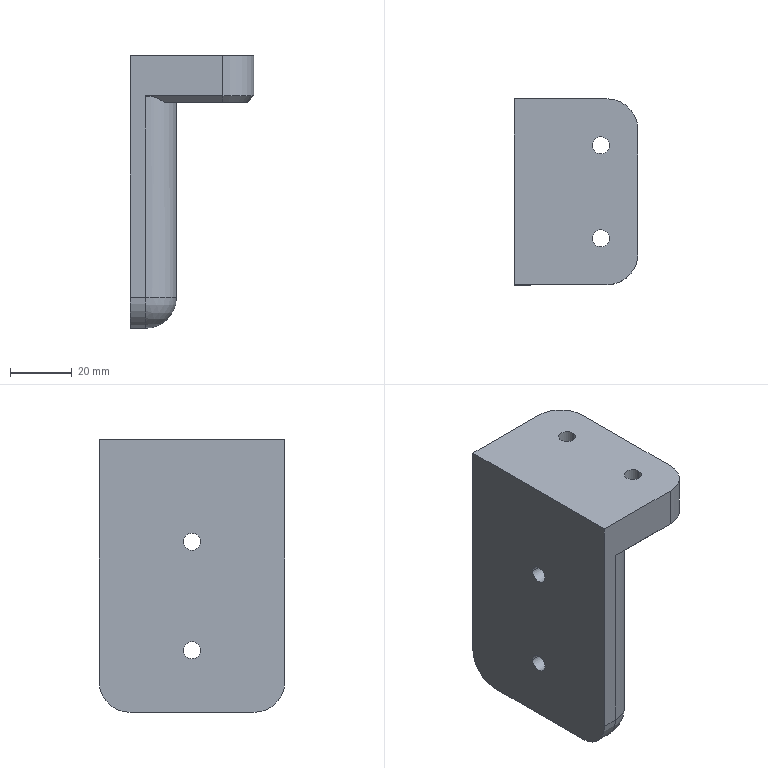Part | NX | features BREP 1 | 1 solid | 42 faces | box 40 x 60 x 88 mm | volume 93544 mm3 | cylinder 23 | plane 15 | cone 2 | sphere 2 | commonest cylinder face diameters 5.5 x8 9.5 x8 20 x7
STEP:
#1=CARTESIAN_POINT('',(30.,0.,-13.));
#2=VERTEX_POINT('',#1);
#3=CARTESIAN_POINT('',(30.,0.,0.));
#4=VERTEX_POINT('',#3);
#5=CARTESIAN_POINT('',(30.,0.,-13.));
#6=DIRECTION('',(0.000000001,0.,1.));
#7=VECTOR('',#6,1000.);
#8=LINE('',#5,#7);
#9=EDGE_CURVE('',#2,#4,#8,.T.);
#10=ORIENTED_EDGE('',*,*,#9,.T.);
#11=CARTESIAN_POINT('',(0.,0.,0.));
#12=VERTEX_POINT('',#11);
#13=CARTESIAN_POINT('',(0.,0.,0.));
#14=DIRECTION('',(1.,0.,0.));
#15=VECTOR('',#14,1000.);
#16=LINE('',#13,#15);
#17=EDGE_CURVE('',#12,#4,#16,.T.);
#18=ORIENTED_EDGE('',*,*,#17,.F.);
#19=CARTESIAN_POINT('',(0.,0.,-78.));
#20=VERTEX_POINT('',#19);
#21=CARTESIAN_POINT('',(0.,0.,-78.));
#22=DIRECTION('',(0.,0.,1.));
#23=VECTOR('',#22,1000.);
#24=LINE('',#21,#23);
#25=EDGE_CURVE('',#20,#12,#24,.T.);
#26=ORIENTED_EDGE('',*,*,#25,.F.);
#27=CARTESIAN_POINT('',(5.,0.,-78.));
#28=VERTEX_POINT('',#27);
#29=CARTESIAN_POINT('',(0.,0.,-78.));
#30=DIRECTION('',(1.,0.,0.));
#31=VECTOR('',#30,1000.);
#32=LINE('',#29,#31);
#33=EDGE_CURVE('',#20,#28,#32,.T.);
#34=ORIENTED_EDGE('',*,*,#33,.T.);
#35=CARTESIAN_POINT('',(5.,0.,-13.));
#36=VERTEX_POINT('',#35);
#37=CARTESIAN_POINT('',(5.,0.,-78.));
#38=DIRECTION('',(0.,0.,1.));
#39=VECTOR('',#38,1000.);
#40=LINE('',#37,#39);
#41=EDGE_CURVE('',#28,#36,#40,.T.);
#42=ORIENTED_EDGE('',*,*,#41,.T.);
#43=CARTESIAN_POINT('',(30.,0.,-13.));
#44=DIRECTION('',(-1.,0.,0.));
#45=VECTOR('',#44,1000.);
#46=LINE('',#43,#45);
#47=EDGE_CURVE('',#2,#36,#46,.T.);
#48=ORIENTED_EDGE('',*,*,#47,.F.);
#49=EDGE_LOOP('',(#10,#18,#26,#34,#42,#48));
#50=FACE_BOUND('',#49,.T.);
#51=CARTESIAN_POINT('',(0.,0.,0.));
#52=DIRECTION('',(0.,1.,0.));
#53=DIRECTION('',(1.,0.,0.));
#54=AXIS2_PLACEMENT_3D('',#51,#52,#53);
#55=PLANE('',#54);
#56=ADVANCED_FACE('',(#50),#55,.F.);
#57=CARTESIAN_POINT('',(11.,2.,-15.));
#58=VERTEX_POINT('',#57);
#59=CARTESIAN_POINT('',(5.,0.,-13.));
#60=CARTESIAN_POINT('',(6.09,0.,-13.));
#61=CARTESIAN_POINT('',(8.347,0.3927,-13.393));
#62=CARTESIAN_POINT('',(10.155,1.366,-14.366));
#63=CARTESIAN_POINT('',(11.,2.,-15.));
#64=B_SPLINE_CURVE_WITH_KNOTS('',3,(#59,#60,#61,#62,#63),.UNSPECIFIED.,.F.,.F.,(4,1,4),(0.,0.5,1.),.UNSPECIFIED.);
#65=EDGE_CURVE('',#58,#36,#64,.F.);
#66=ORIENTED_EDGE('',*,*,#65,.F.);
#67=CARTESIAN_POINT('',(30.,2.,-15.));
#68=VERTEX_POINT('',#67);
#69=CARTESIAN_POINT('',(30.,2.,-15.));
#70=DIRECTION('',(-1.,0.,0.));
#71=VECTOR('',#70,1000.);
#72=LINE('',#69,#71);
#73=EDGE_CURVE('',#68,#58,#72,.T.);
#74=ORIENTED_EDGE('',*,*,#73,.F.);
#75=CARTESIAN_POINT('',(30.,2.,-15.));
#76=DIRECTION('',(0.,-0.7071,0.7071));
#77=VECTOR('',#76,1000.);
#78=LINE('',#75,#77);
#79=EDGE_CURVE('',#68,#2,#78,.T.);
#80=ORIENTED_EDGE('',*,*,#79,.T.);
#81=ORIENTED_EDGE('',*,*,#47,.T.);
#82=EDGE_LOOP('',(#66,#74,#80,#81));
#83=FACE_BOUND('',#82,.T.);
#84=CARTESIAN_POINT('',(20.5,1.,-14.));
#85=DIRECTION('',(0.,-0.7071,-0.7071));
#86=DIRECTION('',(0.,-0.7071,0.7071));
#87=AXIS2_PLACEMENT_3D('',#84,#85,#86);
#88=PLANE('',#87);
#89=ADVANCED_FACE('',(#83),#88,.T.);
#90=CARTESIAN_POINT('',(38.,10.,-15.));
#91=VERTEX_POINT('',#90);
#92=CARTESIAN_POINT('',(40.,10.,-13.));
#93=VERTEX_POINT('',#92);
#94=CARTESIAN_POINT('',(38.,10.,-15.));
#95=DIRECTION('',(0.7071,0.,0.7071));
#96=VECTOR('',#95,1000.);
#97=LINE('',#94,#96);
#98=EDGE_CURVE('',#91,#93,#97,.T.);
#99=ORIENTED_EDGE('',*,*,#98,.T.);
#100=CARTESIAN_POINT('',(30.,10.,-13.));
#101=DIRECTION('',(0.,0.,-1.));
#102=DIRECTION('',(1.,0.,0.));
#103=AXIS2_PLACEMENT_3D('',#100,#101,#102);
#104=CIRCLE('',#103,10.);
#105=EDGE_CURVE('',#93,#2,#104,.T.);
#106=ORIENTED_EDGE('',*,*,#105,.T.);
#107=ORIENTED_EDGE('',*,*,#79,.F.);
#108=CARTESIAN_POINT('',(30.,10.,-15.));
#109=DIRECTION('',(0.,0.,-1.));
#110=DIRECTION('',(1.,0.,0.));
#111=AXIS2_PLACEMENT_3D('',#108,#109,#110);
#112=CIRCLE('',#111,8.);
#113=EDGE_CURVE('',#91,#68,#112,.T.);
#114=ORIENTED_EDGE('',*,*,#113,.F.);
#115=EDGE_LOOP('',(#99,#106,#107,#114));
#116=FACE_BOUND('',#115,.T.);
#117=CARTESIAN_POINT('',(30.,10.,-14.));
#118=DIRECTION('',(0.,0.,1.));
#119=DIRECTION('',(0.,-1.,0.));
#120=AXIS2_PLACEMENT_3D('',#117,#118,#119);
#121=CONICAL_SURFACE('',#120,9.,0.7854);
#122=ADVANCED_FACE('',(#116),#121,.T.);
#123=CARTESIAN_POINT('',(15.,10.,-15.));
#124=VERTEX_POINT('',#123);
#125=CARTESIAN_POINT('',(5.,10.,-15.));
#126=DIRECTION('',(0.,0.,1.));
#127=DIRECTION('',(0.6,-0.8,0.));
#128=AXIS2_PLACEMENT_3D('',#125,#126,#127);
#129=CIRCLE('',#128,10.);
#130=EDGE_CURVE('',#58,#124,#129,.T.);
#131=ORIENTED_EDGE('',*,*,#130,.T.);
#132=CARTESIAN_POINT('',(15.,50.,-15.));
#133=VERTEX_POINT('',#132);
#134=CARTESIAN_POINT('',(15.,10.,-15.));
#135=DIRECTION('',(0.,1.,0.));
#136=VECTOR('',#135,1000.);
#137=LINE('',#134,#136);
#138=EDGE_CURVE('',#124,#133,#137,.T.);
#139=ORIENTED_EDGE('',*,*,#138,.T.);
#140=CARTESIAN_POINT('',(11.,58.,-15.));
#141=VERTEX_POINT('',#140);
#142=CARTESIAN_POINT('',(5.,50.,-15.));
#143=DIRECTION('',(0.,0.,1.));
#144=DIRECTION('',(1.,0.,0.));
#145=AXIS2_PLACEMENT_3D('',#142,#143,#144);
#146=CIRCLE('',#145,10.);
#147=EDGE_CURVE('',#133,#141,#146,.T.);
#148=ORIENTED_EDGE('',*,*,#147,.T.);
#149=CARTESIAN_POINT('',(30.,58.,-15.));
#150=VERTEX_POINT('',#149);
#151=CARTESIAN_POINT('',(11.,58.,-15.));
#152=DIRECTION('',(1.,0.,0.));
#153=VECTOR('',#152,1000.);
#154=LINE('',#151,#153);
#155=EDGE_CURVE('',#141,#150,#154,.T.);
#156=ORIENTED_EDGE('',*,*,#155,.T.);
#157=CARTESIAN_POINT('',(38.,50.,-15.));
#158=VERTEX_POINT('',#157);
#159=CARTESIAN_POINT('',(30.,50.,-15.));
#160=DIRECTION('',(0.,0.,-1.));
#161=DIRECTION('',(0.,1.,0.));
#162=AXIS2_PLACEMENT_3D('',#159,#160,#161);
#163=CIRCLE('',#162,8.);
#164=EDGE_CURVE('',#150,#158,#163,.T.);
#165=ORIENTED_EDGE('',*,*,#164,.T.);
#166=CARTESIAN_POINT('',(38.,50.,-15.));
#167=DIRECTION('',(0.,-1.,0.));
#168=VECTOR('',#167,1000.);
#169=LINE('',#166,#168);
#170=EDGE_CURVE('',#158,#91,#169,.T.);
#171=ORIENTED_EDGE('',*,*,#170,.T.);
#172=ORIENTED_EDGE('',*,*,#113,.T.);
#173=ORIENTED_EDGE('',*,*,#73,.T.);
#174=EDGE_LOOP('',(#131,#139,#148,#156,#165,#171,#172,#173));
#175=FACE_BOUND('',#174,.T.);
#176=CARTESIAN_POINT('',(23.25,45.,-15.));
#177=VERTEX_POINT('',#176);
#178=CARTESIAN_POINT('',(32.75,45.,-15.));
#179=VERTEX_POINT('',#178);
#180=CARTESIAN_POINT('',(28.,45.,-15.));
#181=DIRECTION('',(0.,0.,-1.));
#182=DIRECTION('',(-1.,0.,0.));
#183=AXIS2_PLACEMENT_3D('',#180,#181,#182);
#184=CIRCLE('',#183,4.75);
#185=EDGE_CURVE('',#177,#179,#184,.T.);
#186=ORIENTED_EDGE('',*,*,#185,.F.);
#187=CARTESIAN_POINT('',(28.,45.,-15.));
#188=DIRECTION('',(0.,0.,-1.));
#189=DIRECTION('',(1.,0.,0.));
#190=AXIS2_PLACEMENT_3D('',#187,#188,#189);
#191=CIRCLE('',#190,4.75);
#192=EDGE_CURVE('',#179,#177,#191,.T.);
#193=ORIENTED_EDGE('',*,*,#192,.F.);
#194=EDGE_LOOP('',(#186,#193));
#195=FACE_BOUND('',#194,.T.);
#196=CARTESIAN_POINT('',(23.25,15.,-15.));
#197=VERTEX_POINT('',#196);
#198=CARTESIAN_POINT('',(32.75,15.,-15.));
#199=VERTEX_POINT('',#198);
#200=CARTESIAN_POINT('',(28.,15.,-15.));
#201=DIRECTION('',(0.,0.,-1.));
#202=DIRECTION('',(-1.,0.,0.));
#203=AXIS2_PLACEMENT_3D('',#200,#201,#202);
#204=CIRCLE('',#203,4.75);
#205=EDGE_CURVE('',#197,#199,#204,.T.);
#206=ORIENTED_EDGE('',*,*,#205,.F.);
#207=CARTESIAN_POINT('',(28.,15.,-15.));
#208=DIRECTION('',(0.,0.,-1.));
#209=DIRECTION('',(1.,0.,0.));
#210=AXIS2_PLACEMENT_3D('',#207,#208,#209);
#211=CIRCLE('',#210,4.75);
#212=EDGE_CURVE('',#199,#197,#211,.T.);
#213=ORIENTED_EDGE('',*,*,#212,.F.);
#214=EDGE_LOOP('',(#206,#213));
#215=FACE_BOUND('',#214,.T.);
#216=CARTESIAN_POINT('',(40.,0.,-15.));
#217=DIRECTION('',(0.,0.,-1.));
#218=DIRECTION('',(0.,-1.,0.));
#219=AXIS2_PLACEMENT_3D('',#216,#217,#218);
#220=PLANE('',#219);
#221=ADVANCED_FACE('',(#175,#195,#215),#220,.T.);
#222=CARTESIAN_POINT('',(40.,50.,-13.));
#223=VERTEX_POINT('',#222);
#224=CARTESIAN_POINT('',(38.,50.,-15.));
#225=DIRECTION('',(0.7071,0.,0.7071));
#226=VECTOR('',#225,1000.);
#227=LINE('',#224,#226);
#228=EDGE_CURVE('',#158,#223,#227,.T.);
#229=ORIENTED_EDGE('',*,*,#228,.T.);
#230=CARTESIAN_POINT('',(40.,50.,-13.));
#231=DIRECTION('',(0.,-1.,0.));
#232=VECTOR('',#231,1000.);
#233=LINE('',#230,#232);
#234=EDGE_CURVE('',#223,#93,#233,.T.);
#235=ORIENTED_EDGE('',*,*,#234,.T.);
#236=ORIENTED_EDGE('',*,*,#98,.F.);
#237=ORIENTED_EDGE('',*,*,#170,.F.);
#238=EDGE_LOOP('',(#229,#235,#236,#237));
#239=FACE_BOUND('',#238,.T.);
#240=CARTESIAN_POINT('',(39.,30.,-14.));
#241=DIRECTION('',(0.7071,0.,-0.7071));
#242=DIRECTION('',(0.,-1.,0.));
#243=AXIS2_PLACEMENT_3D('',#240,#241,#242);
#244=PLANE('',#243);
#245=ADVANCED_FACE('',(#239),#244,.T.);
#246=CARTESIAN_POINT('',(40.,50.,0.));
#247=VERTEX_POINT('',#246);
#248=CARTESIAN_POINT('',(40.,50.,0.));
#249=DIRECTION('',(0.,-0.000000001,-1.));
#250=VECTOR('',#249,1000.);
#251=LINE('',#248,#250);
#252=EDGE_CURVE('',#247,#223,#251,.T.);
#253=ORIENTED_EDGE('',*,*,#252,.F.);
#254=CARTESIAN_POINT('',(40.,10.,0.));
#255=VERTEX_POINT('',#254);
#256=CARTESIAN_POINT('',(40.,10.,0.));
#257=DIRECTION('',(0.,1.,0.));
#258=VECTOR('',#257,1000.);
#259=LINE('',#256,#258);
#260=EDGE_CURVE('',#255,#247,#259,.T.);
#261=ORIENTED_EDGE('',*,*,#260,.F.);
#262=CARTESIAN_POINT('',(40.,10.,-13.));
#263=DIRECTION('',(0.,-0.000000001,1.));
#264=VECTOR('',#263,1000.);
#265=LINE('',#262,#264);
#266=EDGE_CURVE('',#93,#255,#265,.T.);
#267=ORIENTED_EDGE('',*,*,#266,.F.);
#268=ORIENTED_EDGE('',*,*,#234,.F.);
#269=EDGE_LOOP('',(#253,#261,#267,#268));
#270=FACE_BOUND('',#269,.T.);
#271=CARTESIAN_POINT('',(40.,0.,0.));
#272=DIRECTION('',(1.,0.,0.));
#273=DIRECTION('',(0.,1.,0.));
#274=AXIS2_PLACEMENT_3D('',#271,#272,#273);
#275=PLANE('',#274);
#276=ADVANCED_FACE('',(#270),#275,.T.);
#277=ORIENTED_EDGE('',*,*,#266,.T.);
#278=CARTESIAN_POINT('',(30.,10.,0.));
#279=DIRECTION('',(0.,0.,1.));
#280=DIRECTION('',(0.,-1.,0.));
#281=AXIS2_PLACEMENT_3D('',#278,#279,#280);
#282=CIRCLE('',#281,10.);
#283=EDGE_CURVE('',#4,#255,#282,.T.);
#284=ORIENTED_EDGE('',*,*,#283,.F.);
#285=ORIENTED_EDGE('',*,*,#9,.F.);
#286=ORIENTED_EDGE('',*,*,#105,.F.);
#287=EDGE_LOOP('',(#277,#284,#285,#286));
#288=FACE_BOUND('',#287,.T.);
#289=CARTESIAN_POINT('',(30.,10.,-202.717));
#290=DIRECTION('',(0.,0.,1.));
#291=DIRECTION('',(0.,-1.,0.));
#292=AXIS2_PLACEMENT_3D('',#289,#290,#291);
#293=CYLINDRICAL_SURFACE('',#292,10.);
#294=ADVANCED_FACE('',(#288),#293,.T.);
#295=CARTESIAN_POINT('',(0.,60.,0.));
#296=VERTEX_POINT('',#295);
#297=CARTESIAN_POINT('',(30.,60.,0.));
#298=VERTEX_POINT('',#297);
#299=CARTESIAN_POINT('',(0.,60.,0.));
#300=DIRECTION('',(1.,0.,0.));
#301=VECTOR('',#300,1000.);
#302=LINE('',#299,#301);
#303=EDGE_CURVE('',#296,#298,#302,.T.);
#304=ORIENTED_EDGE('',*,*,#303,.F.);
#305=CARTESIAN_POINT('',(0.,0.,0.));
#306=DIRECTION('',(0.,1.,0.));
#307=VECTOR('',#306,1000.);
#308=LINE('',#305,#307);
#309=EDGE_CURVE('',#12,#296,#308,.T.);
#310=ORIENTED_EDGE('',*,*,#309,.F.);
#311=ORIENTED_EDGE('',*,*,#17,.T.);
#312=ORIENTED_EDGE('',*,*,#283,.T.);
#313=ORIENTED_EDGE('',*,*,#260,.T.);
#314=CARTESIAN_POINT('',(30.,50.,0.));
#315=DIRECTION('',(0.,0.,1.));
#316=DIRECTION('',(1.,0.,0.));
#317=AXIS2_PLACEMENT_3D('',#314,#315,#316);
#318=CIRCLE('',#317,10.);
#319=EDGE_CURVE('',#247,#298,#318,.T.);
#320=ORIENTED_EDGE('',*,*,#319,.T.);
#321=EDGE_LOOP('',(#304,#310,#311,#312,#313,#320));
#322=FACE_BOUND('',#321,.T.);
#323=CARTESIAN_POINT('',(25.25,45.,0.));
#324=VERTEX_POINT('',#323);
#325=CARTESIAN_POINT('',(30.75,45.,0.));
#326=VERTEX_POINT('',#325);
#327=CARTESIAN_POINT('',(28.,45.,0.));
#328=DIRECTION('',(0.,0.,-1.));
#329=DIRECTION('',(-1.,0.,0.));
#330=AXIS2_PLACEMENT_3D('',#327,#328,#329);
#331=CIRCLE('',#330,2.75);
#332=EDGE_CURVE('',#324,#326,#331,.T.);
#333=ORIENTED_EDGE('',*,*,#332,.T.);
#334=CARTESIAN_POINT('',(28.,45.,0.));
#335=DIRECTION('',(0.,0.,-1.));
#336=DIRECTION('',(1.,0.,0.));
#337=AXIS2_PLACEMENT_3D('',#334,#335,#336);
#338=CIRCLE('',#337,2.75);
#339=EDGE_CURVE('',#326,#324,#338,.T.);
#340=ORIENTED_EDGE('',*,*,#339,.T.);
#341=EDGE_LOOP('',(#333,#340));
#342=FACE_BOUND('',#341,.T.);
#343=CARTESIAN_POINT('',(25.25,15.,0.));
#344=VERTEX_POINT('',#343);
#345=CARTESIAN_POINT('',(30.75,15.,0.));
#346=VERTEX_POINT('',#345);
#347=CARTESIAN_POINT('',(28.,15.,0.));
#348=DIRECTION('',(0.,0.,-1.));
#349=DIRECTION('',(-1.,0.,0.));
#350=AXIS2_PLACEMENT_3D('',#347,#348,#349);
#351=CIRCLE('',#350,2.75);
#352=EDGE_CURVE('',#344,#346,#351,.T.);
#353=ORIENTED_EDGE('',*,*,#352,.T.);
#354=CARTESIAN_POINT('',(28.,15.,0.));
#355=DIRECTION('',(0.,0.,-1.));
#356=DIRECTION('',(1.,0.,0.));
#357=AXIS2_PLACEMENT_3D('',#354,#355,#356);
#358=CIRCLE('',#357,2.75);
#359=EDGE_CURVE('',#346,#344,#358,.T.);
#360=ORIENTED_EDGE('',*,*,#359,.T.);
#361=EDGE_LOOP('',(#353,#360));
#362=FACE_BOUND('',#361,.T.);
#363=CARTESIAN_POINT('',(0.,0.,0.));
#364=DIRECTION('',(0.,0.,1.));
#365=DIRECTION('',(1.,0.,0.));
#366=AXIS2_PLACEMENT_3D('',#363,#364,#365);
#367=PLANE('',#366);
#368=ADVANCED_FACE('',(#322,#342,#362),#367,.T.);
#369=CARTESIAN_POINT('',(30.,60.,-13.));
#370=VERTEX_POINT('',#369);
#371=CARTESIAN_POINT('',(30.,60.,0.));
#372=DIRECTION('',(-0.000000001,0.,-1.));
#373=VECTOR('',#372,1000.);
#374=LINE('',#371,#373);
#375=EDGE_CURVE('',#298,#370,#374,.T.);
#376=ORIENTED_EDGE('',*,*,#375,.F.);
#377=ORIENTED_EDGE('',*,*,#319,.F.);
#378=ORIENTED_EDGE('',*,*,#252,.T.);
#379=CARTESIAN_POINT('',(30.,50.,-13.));
#380=DIRECTION('',(0.,0.,-1.));
#381=DIRECTION('',(0.,1.,0.));
#382=AXIS2_PLACEMENT_3D('',#379,#380,#381);
#383=CIRCLE('',#382,10.);
#384=EDGE_CURVE('',#370,#223,#383,.T.);
#385=ORIENTED_EDGE('',*,*,#384,.F.);
#386=EDGE_LOOP('',(#376,#377,#378,#385));
#387=FACE_BOUND('',#386,.T.);
#388=CARTESIAN_POINT('',(30.,50.,114.717));
#389=DIRECTION('',(0.,0.,-1.));
#390=DIRECTION('',(0.,1.,0.));
#391=AXIS2_PLACEMENT_3D('',#388,#389,#390);
#392=CYLINDRICAL_SURFACE('',#391,10.);
#393=ADVANCED_FACE('',(#387),#392,.T.);
#394=CARTESIAN_POINT('',(30.,58.,-15.));
#395=DIRECTION('',(0.,0.7071,0.7071));
#396=VECTOR('',#395,1000.);
#397=LINE('',#394,#396);
#398=EDGE_CURVE('',#150,#370,#397,.T.);
#399=ORIENTED_EDGE('',*,*,#398,.T.);
#400=ORIENTED_EDGE('',*,*,#384,.T.);
#401=ORIENTED_EDGE('',*,*,#228,.F.);
#402=ORIENTED_EDGE('',*,*,#164,.F.);
#403=EDGE_LOOP('',(#399,#400,#401,#402));
#404=FACE_BOUND('',#403,.T.);
#405=CARTESIAN_POINT('',(30.,50.,-14.));
#406=DIRECTION('',(0.,0.,1.));
#407=DIRECTION('',(0.,-1.,0.));
#408=AXIS2_PLACEMENT_3D('',#405,#406,#407);
#409=CONICAL_SURFACE('',#408,9.,0.7854);
#410=ADVANCED_FACE('',(#404),#409,.T.);
#411=CARTESIAN_POINT('',(5.,60.,-13.));
#412=VERTEX_POINT('',#411);
#413=CARTESIAN_POINT('',(11.,58.,-15.));
#414=CARTESIAN_POINT('',(10.166,58.626,-14.374));
#415=CARTESIAN_POINT('',(8.361,59.604,-13.396));
#416=CARTESIAN_POINT('',(6.096,60.,-13.));
#417=CARTESIAN_POINT('',(5.,60.,-13.));
#418=B_SPLINE_CURVE_WITH_KNOTS('',3,(#413,#414,#415,#416,#417),.UNSPECIFIED.,.F.,.F.,(4,1,4),(0.,0.5,1.),.UNSPECIFIED.);
#419=EDGE_CURVE('',#412,#141,#418,.F.);
#420=ORIENTED_EDGE('',*,*,#419,.F.);
#421=CARTESIAN_POINT('',(5.,60.,-13.));
#422=DIRECTION('',(1.,0.,0.));
#423=VECTOR('',#422,1000.);
#424=LINE('',#421,#423);
#425=EDGE_CURVE('',#412,#370,#424,.T.);
#426=ORIENTED_EDGE('',*,*,#425,.T.);
#427=ORIENTED_EDGE('',*,*,#398,.F.);
#428=ORIENTED_EDGE('',*,*,#155,.F.);
#429=EDGE_LOOP('',(#420,#426,#427,#428));
#430=FACE_BOUND('',#429,.T.);
#431=CARTESIAN_POINT('',(20.5,59.,-14.));
#432=DIRECTION('',(0.,0.7071,-0.7071));
#433=DIRECTION('',(-1.,0.,0.));
#434=AXIS2_PLACEMENT_3D('',#431,#432,#433);
#435=PLANE('',#434);
#436=ADVANCED_FACE('',(#430),#435,.T.);
#437=CARTESIAN_POINT('',(5.,60.,-78.));
#438=VERTEX_POINT('',#437);
#439=CARTESIAN_POINT('',(5.,60.,-13.));
#440=DIRECTION('',(0.,0.,-1.));
#441=VECTOR('',#440,1000.);
#442=LINE('',#439,#441);
#443=EDGE_CURVE('',#412,#438,#442,.T.);
#444=ORIENTED_EDGE('',*,*,#443,.T.);
#445=CARTESIAN_POINT('',(0.,60.,-78.));
#446=VERTEX_POINT('',#445);
#447=CARTESIAN_POINT('',(5.,60.,-78.));
#448=DIRECTION('',(-1.,0.,0.));
#449=VECTOR('',#448,1000.);
#450=LINE('',#447,#449);
#451=EDGE_CURVE('',#438,#446,#450,.T.);
#452=ORIENTED_EDGE('',*,*,#451,.T.);
#453=CARTESIAN_POINT('',(0.,60.,-78.));
#454=DIRECTION('',(0.,0.,1.));
#455=VECTOR('',#454,1000.);
#456=LINE('',#453,#455);
#457=EDGE_CURVE('',#446,#296,#456,.T.);
#458=ORIENTED_EDGE('',*,*,#457,.T.);
#459=ORIENTED_EDGE('',*,*,#303,.T.);
#460=ORIENTED_EDGE('',*,*,#375,.T.);
#461=ORIENTED_EDGE('',*,*,#425,.F.);
#462=EDGE_LOOP('',(#444,#452,#458,#459,#460,#461));
#463=FACE_BOUND('',#462,.T.);
#464=CARTESIAN_POINT('',(0.,60.,0.));
#465=DIRECTION('',(0.,1.,0.));
#466=DIRECTION('',(1.,0.,0.));
#467=AXIS2_PLACEMENT_3D('',#464,#465,#466);
#468=PLANE('',#467);
#469=ADVANCED_FACE('',(#463),#468,.T.);
#470=CARTESIAN_POINT('',(0.,10.,-88.));
#471=VERTEX_POINT('',#470);
#472=CARTESIAN_POINT('',(0.,50.,-88.));
#473=VERTEX_POINT('',#472);
#474=CARTESIAN_POINT('',(0.,10.,-88.));
#475=DIRECTION('',(0.,1.,0.));
#476=VECTOR('',#475,1000.);
#477=LINE('',#474,#476);
#478=EDGE_CURVE('',#471,#473,#477,.T.);
#479=ORIENTED_EDGE('',*,*,#478,.F.);
#480=CARTESIAN_POINT('',(0.,10.,-78.));
#481=DIRECTION('',(-1.,0.,0.));
#482=DIRECTION('',(0.,0.,-1.));
#483=AXIS2_PLACEMENT_3D('',#480,#481,#482);
#484=CIRCLE('',#483,10.);
#485=EDGE_CURVE('',#471,#20,#484,.T.);
#486=ORIENTED_EDGE('',*,*,#485,.T.);
#487=ORIENTED_EDGE('',*,*,#25,.T.);
#488=ORIENTED_EDGE('',*,*,#309,.T.);
#489=ORIENTED_EDGE('',*,*,#457,.F.);
#490=CARTESIAN_POINT('',(0.,50.,-78.));
#491=DIRECTION('',(-1.,0.,0.));
#492=DIRECTION('',(0.,1.,0.));
#493=AXIS2_PLACEMENT_3D('',#490,#491,#492);
#494=CIRCLE('',#493,10.);
#495=EDGE_CURVE('',#446,#473,#494,.T.);
#496=ORIENTED_EDGE('',*,*,#495,.T.);
#497=EDGE_LOOP('',(#479,#486,#487,#488,#489,#496));
#498=FACE_BOUND('',#497,.T.);
#499=CARTESIAN_POINT('',(0.,32.75,-68.));
#500=VERTEX_POINT('',#499);
#501=CARTESIAN_POINT('',(0.,27.25,-68.));
#502=VERTEX_POINT('',#501);
#503=CARTESIAN_POINT('',(0.,30.,-68.));
#504=DIRECTION('',(1.,0.,0.));
#505=DIRECTION('',(0.,1.,0.));
#506=AXIS2_PLACEMENT_3D('',#503,#504,#505);
#507=CIRCLE('',#506,2.75);
#508=EDGE_CURVE('',#500,#502,#507,.T.);
#509=ORIENTED_EDGE('',*,*,#508,.T.);
#510=CARTESIAN_POINT('',(0.,30.,-68.));
#511=DIRECTION('',(1.,0.,0.));
#512=DIRECTION('',(0.,-1.,0.));
#513=AXIS2_PLACEMENT_3D('',#510,#511,#512);
#514=CIRCLE('',#513,2.75);
#515=EDGE_CURVE('',#502,#500,#514,.T.);
#516=ORIENTED_EDGE('',*,*,#515,.T.);
#517=EDGE_LOOP('',(#509,#516));
#518=FACE_BOUND('',#517,.T.);
#519=CARTESIAN_POINT('',(0.,32.75,-33.));
#520=VERTEX_POINT('',#519);
#521=CARTESIAN_POINT('',(0.,27.25,-33.));
#522=VERTEX_POINT('',#521);
#523=CARTESIAN_POINT('',(0.,30.,-33.));
#524=DIRECTION('',(1.,0.,0.));
#525=DIRECTION('',(0.,1.,0.));
#526=AXIS2_PLACEMENT_3D('',#523,#524,#525);
#527=CIRCLE('',#526,2.75);
#528=EDGE_CURVE('',#520,#522,#527,.T.);
#529=ORIENTED_EDGE('',*,*,#528,.T.);
#530=CARTESIAN_POINT('',(0.,30.,-33.));
#531=DIRECTION('',(1.,0.,0.));
#532=DIRECTION('',(0.,-1.,0.));
#533=AXIS2_PLACEMENT_3D('',#530,#531,#532);
#534=CIRCLE('',#533,2.75);
#535=EDGE_CURVE('',#522,#520,#534,.T.);
#536=ORIENTED_EDGE('',*,*,#535,.T.);
#537=EDGE_LOOP('',(#529,#536));
#538=FACE_BOUND('',#537,.T.);
#539=CARTESIAN_POINT('',(0.,0.,-88.));
#540=DIRECTION('',(-1.,0.,0.));
#541=DIRECTION('',(0.,0.,1.));
#542=AXIS2_PLACEMENT_3D('',#539,#540,#541);
#543=PLANE('',#542);
#544=ADVANCED_FACE('',(#498,#518,#538),#543,.T.);
#545=ORIENTED_EDGE('',*,*,#451,.F.);
#546=CARTESIAN_POINT('',(5.,50.,-88.));
#547=VERTEX_POINT('',#546);
#548=CARTESIAN_POINT('',(5.,50.,-78.));
#549=DIRECTION('',(-1.,0.,0.));
#550=DIRECTION('',(0.,1.,0.));
#551=AXIS2_PLACEMENT_3D('',#548,#549,#550);
#552=CIRCLE('',#551,10.);
#553=EDGE_CURVE('',#438,#547,#552,.T.);
#554=ORIENTED_EDGE('',*,*,#553,.T.);
#555=CARTESIAN_POINT('',(5.,50.,-88.));
#556=DIRECTION('',(-1.,0.,0.));
#557=VECTOR('',#556,1000.);
#558=LINE('',#555,#557);
#559=EDGE_CURVE('',#547,#473,#558,.T.);
#560=ORIENTED_EDGE('',*,*,#559,.T.);
#561=ORIENTED_EDGE('',*,*,#495,.F.);
#562=EDGE_LOOP('',(#545,#554,#560,#561));
#563=FACE_BOUND('',#562,.T.);
#564=CARTESIAN_POINT('',(15.175,50.,-78.));
#565=DIRECTION('',(-1.,0.,0.));
#566=DIRECTION('',(0.,1.,0.));
#567=AXIS2_PLACEMENT_3D('',#564,#565,#566);
#568=CYLINDRICAL_SURFACE('',#567,10.);
#569=ADVANCED_FACE('',(#563),#568,.T.);
#570=CARTESIAN_POINT('',(5.,10.,-88.));
#571=VERTEX_POINT('',#570);
#572=CARTESIAN_POINT('',(5.,10.,-88.));
#573=DIRECTION('',(0.,1.,0.));
#574=VECTOR('',#573,1000.);
#575=LINE('',#572,#574);
#576=EDGE_CURVE('',#571,#547,#575,.T.);
#577=ORIENTED_EDGE('',*,*,#576,.F.);
#578=CARTESIAN_POINT('',(0.,10.,-88.));
#579=DIRECTION('',(1.,0.,0.));
#580=VECTOR('',#579,1000.);
#581=LINE('',#578,#580);
#582=EDGE_CURVE('',#471,#571,#581,.T.);
#583=ORIENTED_EDGE('',*,*,#582,.F.);
#584=ORIENTED_EDGE('',*,*,#478,.T.);
#585=ORIENTED_EDGE('',*,*,#559,.F.);
#586=EDGE_LOOP('',(#577,#583,#584,#585));
#587=FACE_BOUND('',#586,.T.);
#588=CARTESIAN_POINT('',(15.,0.,-88.));
#589=DIRECTION('',(0.,0.,-1.));
#590=DIRECTION('',(0.,-1.,0.));
#591=AXIS2_PLACEMENT_3D('',#588,#589,#590);
#592=PLANE('',#591);
#593=ADVANCED_FACE('',(#587),#592,.T.);
#594=ORIENTED_EDGE('',*,*,#582,.T.);
#595=CARTESIAN_POINT('',(5.,10.,-78.));
#596=DIRECTION('',(1.,0.,0.));
#597=DIRECTION('',(0.,-1.,0.));
#598=AXIS2_PLACEMENT_3D('',#595,#596,#597);
#599=CIRCLE('',#598,10.);
#600=EDGE_CURVE('',#28,#571,#599,.T.);
#601=ORIENTED_EDGE('',*,*,#600,.F.);
#602=ORIENTED_EDGE('',*,*,#33,.F.);
#603=ORIENTED_EDGE('',*,*,#485,.F.);
#604=EDGE_LOOP('',(#594,#601,#602,#603));
#605=FACE_BOUND('',#604,.T.);
#606=CARTESIAN_POINT('',(-52.144,10.,-78.));
#607=DIRECTION('',(1.,0.,0.));
#608=DIRECTION('',(0.,-1.,0.));
#609=AXIS2_PLACEMENT_3D('',#606,#607,#608);
#610=CYLINDRICAL_SURFACE('',#609,10.);
#611=ADVANCED_FACE('',(#605),#610,.T.);
#612=ORIENTED_EDGE('',*,*,#600,.T.);
#613=CARTESIAN_POINT('',(15.,10.,-78.));
#614=VERTEX_POINT('',#613);
#615=CARTESIAN_POINT('',(5.,10.,-78.));
#616=DIRECTION('',(0.,1.,0.));
#617=DIRECTION('',(1.,0.,0.));
#618=AXIS2_PLACEMENT_3D('',#615,#616,#617);
#619=CIRCLE('',#618,10.);
#620=EDGE_CURVE('',#614,#571,#619,.T.);
#621=ORIENTED_EDGE('',*,*,#620,.F.);
#622=CARTESIAN_POINT('',(5.,10.,-78.));
#623=DIRECTION('',(0.,0.,1.));
#624=DIRECTION('',(0.,-1.,0.));
#625=AXIS2_PLACEMENT_3D('',#622,#623,#624);
#626=CIRCLE('',#625,10.);
#627=EDGE_CURVE('',#28,#614,#626,.T.);
#628=ORIENTED_EDGE('',*,*,#627,.F.);
#629=EDGE_LOOP('',(#612,#621,#628));
#630=FACE_BOUND('',#629,.T.);
#631=CARTESIAN_POINT('',(5.,10.,-78.));
#632=DIRECTION('',(0.,0.,1.));
#633=DIRECTION('',(0.7071,-0.7071,0.));
#634=AXIS2_PLACEMENT_3D('',#631,#632,#633);
#635=SPHERICAL_SURFACE('',#634,10.);
#636=ADVANCED_FACE('',(#630),#635,.T.);
#637=ORIENTED_EDGE('',*,*,#627,.T.);
#638=CARTESIAN_POINT('',(15.,10.,-78.));
#639=DIRECTION('',(0.,0.,1.));
#640=VECTOR('',#639,1000.);
#641=LINE('',#638,#640);
#642=EDGE_CURVE('',#614,#124,#641,.T.);
#643=ORIENTED_EDGE('',*,*,#642,.T.);
#644=ORIENTED_EDGE('',*,*,#130,.F.);
#645=ORIENTED_EDGE('',*,*,#65,.T.);
#646=ORIENTED_EDGE('',*,*,#41,.F.);
#647=EDGE_LOOP('',(#637,#643,#644,#645,#646));
#648=FACE_BOUND('',#647,.T.);
#649=CARTESIAN_POINT('',(5.,10.,-202.717));
#650=DIRECTION('',(0.,0.,1.));
#651=DIRECTION('',(0.,-1.,0.));
#652=AXIS2_PLACEMENT_3D('',#649,#650,#651);
#653=CYLINDRICAL_SURFACE('',#652,10.);
#654=ADVANCED_FACE('',(#648),#653,.T.);
#655=ORIENTED_EDGE('',*,*,#138,.F.);
#656=ORIENTED_EDGE('',*,*,#642,.F.);
#657=CARTESIAN_POINT('',(15.,50.,-78.));
#658=VERTEX_POINT('',#657);
#659=CARTESIAN_POINT('',(15.,10.,-78.));
#660=DIRECTION('',(0.,1.,0.));
#661=VECTOR('',#660,1000.);
#662=LINE('',#659,#661);
#663=EDGE_CURVE('',#614,#658,#662,.T.);
#664=ORIENTED_EDGE('',*,*,#663,.T.);
#665=CARTESIAN_POINT('',(15.,50.,-15.));
#666=DIRECTION('',(0.,0.,-1.));
#667=VECTOR('',#666,1000.);
#668=LINE('',#665,#667);
#669=EDGE_CURVE('',#133,#658,#668,.T.);
#670=ORIENTED_EDGE('',*,*,#669,.F.);
#671=EDGE_LOOP('',(#655,#656,#664,#670));
#672=FACE_BOUND('',#671,.T.);
#673=CARTESIAN_POINT('',(15.,34.75,-68.));
#674=VERTEX_POINT('',#673);
#675=CARTESIAN_POINT('',(15.,25.25,-68.));
#676=VERTEX_POINT('',#675);
#677=CARTESIAN_POINT('',(15.,30.,-68.));
#678=DIRECTION('',(1.,0.,0.));
#679=DIRECTION('',(0.,1.,0.));
#680=AXIS2_PLACEMENT_3D('',#677,#678,#679);
#681=CIRCLE('',#680,4.75);
#682=EDGE_CURVE('',#674,#676,#681,.T.);
#683=ORIENTED_EDGE('',*,*,#682,.F.);
#684=CARTESIAN_POINT('',(15.,30.,-68.));
#685=DIRECTION('',(1.,0.,0.));
#686=DIRECTION('',(0.,-1.,0.));
#687=AXIS2_PLACEMENT_3D('',#684,#685,#686);
#688=CIRCLE('',#687,4.75);
#689=EDGE_CURVE('',#676,#674,#688,.T.);
#690=ORIENTED_EDGE('',*,*,#689,.F.);
#691=EDGE_LOOP('',(#683,#690));
#692=FACE_BOUND('',#691,.T.);
#693=CARTESIAN_POINT('',(15.,34.75,-33.));
#694=VERTEX_POINT('',#693);
#695=CARTESIAN_POINT('',(15.,25.25,-33.));
#696=VERTEX_POINT('',#695);
#697=CARTESIAN_POINT('',(15.,30.,-33.));
#698=DIRECTION('',(1.,0.,0.));
#699=DIRECTION('',(0.,1.,0.));
#700=AXIS2_PLACEMENT_3D('',#697,#698,#699);
#701=CIRCLE('',#700,4.75);
#702=EDGE_CURVE('',#694,#696,#701,.T.);
#703=ORIENTED_EDGE('',*,*,#702,.F.);
#704=CARTESIAN_POINT('',(15.,30.,-33.));
#705=DIRECTION('',(1.,0.,0.));
#706=DIRECTION('',(0.,-1.,0.));
#707=AXIS2_PLACEMENT_3D('',#704,#705,#706);
#708=CIRCLE('',#707,4.75);
#709=EDGE_CURVE('',#696,#694,#708,.T.);
#710=ORIENTED_EDGE('',*,*,#709,.F.);
#711=EDGE_LOOP('',(#703,#710));
#712=FACE_BOUND('',#711,.T.);
#713=CARTESIAN_POINT('',(15.,0.,-15.));
#714=DIRECTION('',(1.,0.,0.));
#715=DIRECTION('',(0.,1.,0.));
#716=AXIS2_PLACEMENT_3D('',#713,#714,#715);
#717=PLANE('',#716);
#718=ADVANCED_FACE('',(#672,#692,#712),#717,.T.);
#719=ORIENTED_EDGE('',*,*,#669,.T.);
#720=CARTESIAN_POINT('',(5.,50.,-78.));
#721=DIRECTION('',(0.,0.,1.));
#722=DIRECTION('',(1.,0.,0.));
#723=AXIS2_PLACEMENT_3D('',#720,#721,#722);
#724=CIRCLE('',#723,10.);
#725=EDGE_CURVE('',#658,#438,#724,.T.);
#726=ORIENTED_EDGE('',*,*,#725,.T.);
#727=ORIENTED_EDGE('',*,*,#443,.F.);
#728=ORIENTED_EDGE('',*,*,#419,.T.);
#729=ORIENTED_EDGE('',*,*,#147,.F.);
#730=EDGE_LOOP('',(#719,#726,#727,#728,#729));
#731=FACE_BOUND('',#730,.T.);
#732=CARTESIAN_POINT('',(5.,50.,114.717));
#733=DIRECTION('',(0.,0.,-1.));
#734=DIRECTION('',(0.,1.,0.));
#735=AXIS2_PLACEMENT_3D('',#732,#733,#734);
#736=CYLINDRICAL_SURFACE('',#735,10.);
#737=ADVANCED_FACE('',(#731),#736,.T.);
#738=CARTESIAN_POINT('',(5.,50.,-78.));
#739=DIRECTION('',(0.,1.,0.));
#740=DIRECTION('',(1.,0.,0.));
#741=AXIS2_PLACEMENT_3D('',#738,#739,#740);
#742=CIRCLE('',#741,10.);
#743=EDGE_CURVE('',#658,#547,#742,.T.);
#744=ORIENTED_EDGE('',*,*,#743,.T.);
#745=ORIENTED_EDGE('',*,*,#553,.F.);
#746=ORIENTED_EDGE('',*,*,#725,.F.);
#747=EDGE_LOOP('',(#744,#745,#746));
#748=FACE_BOUND('',#747,.T.);
#749=CARTESIAN_POINT('',(5.,50.,-78.));
#750=DIRECTION('',(0.,0.,1.));
#751=DIRECTION('',(0.7071,0.7071,0.));
#752=AXIS2_PLACEMENT_3D('',#749,#750,#751);
#753=SPHERICAL_SURFACE('',#752,10.);
#754=ADVANCED_FACE('',(#748),#753,.T.);
#755=ORIENTED_EDGE('',*,*,#620,.T.);
#756=ORIENTED_EDGE('',*,*,#576,.T.);
#757=ORIENTED_EDGE('',*,*,#743,.F.);
#758=ORIENTED_EDGE('',*,*,#663,.F.);
#759=EDGE_LOOP('',(#755,#756,#757,#758));
#760=FACE_BOUND('',#759,.T.);
#761=CARTESIAN_POINT('',(5.,9.828,-78.));
#762=DIRECTION('',(0.,1.,0.));
#763=DIRECTION('',(1.,0.,0.));
#764=AXIS2_PLACEMENT_3D('',#761,#762,#763);
#765=CYLINDRICAL_SURFACE('',#764,10.);
#766=ADVANCED_FACE('',(#760),#765,.T.);
#767=CARTESIAN_POINT('',(9.,34.75,-68.));
#768=VERTEX_POINT('',#767);
#769=CARTESIAN_POINT('',(9.,34.75,-68.));
#770=DIRECTION('',(1.,0.,0.));
#771=VECTOR('',#770,1000.);
#772=LINE('',#769,#771);
#773=EDGE_CURVE('',#674,#768,#772,.F.);
#774=ORIENTED_EDGE('',*,*,#773,.T.);
#775=CARTESIAN_POINT('',(9.,25.25,-68.));
#776=VERTEX_POINT('',#775);
#777=CARTESIAN_POINT('',(9.,30.,-68.));
#778=DIRECTION('',(1.,0.,0.));
#779=DIRECTION('',(0.,-1.,0.));
#780=AXIS2_PLACEMENT_3D('',#777,#778,#779);
#781=CIRCLE('',#780,4.75);
#782=EDGE_CURVE('',#776,#768,#781,.T.);
#783=ORIENTED_EDGE('',*,*,#782,.F.);
#784=CARTESIAN_POINT('',(9.,25.25,-68.));
#785=DIRECTION('',(1.,0.,0.));
#786=VECTOR('',#785,1000.);
#787=LINE('',#784,#786);
#788=EDGE_CURVE('',#676,#776,#787,.F.);
#789=ORIENTED_EDGE('',*,*,#788,.F.);
#790=ORIENTED_EDGE('',*,*,#689,.T.);
#791=EDGE_LOOP('',(#774,#783,#789,#790));
#792=FACE_BOUND('',#791,.T.);
#793=CARTESIAN_POINT('',(-16.597,30.,-68.));
#794=DIRECTION('',(1.,0.,0.));
#795=DIRECTION('',(0.,-1.,0.));
#796=AXIS2_PLACEMENT_3D('',#793,#794,#795);
#797=CYLINDRICAL_SURFACE('',#796,4.75);
#798=ADVANCED_FACE('',(#792),#797,.F.);
#799=ORIENTED_EDGE('',*,*,#788,.T.);
#800=CARTESIAN_POINT('',(9.,30.,-68.));
#801=DIRECTION('',(-1.,0.,0.));
#802=DIRECTION('',(0.,-1.,0.));
#803=AXIS2_PLACEMENT_3D('',#800,#801,#802);
#804=CIRCLE('',#803,4.75);
#805=EDGE_CURVE('',#776,#768,#804,.T.);
#806=ORIENTED_EDGE('',*,*,#805,.T.);
#807=ORIENTED_EDGE('',*,*,#773,.F.);
#808=ORIENTED_EDGE('',*,*,#682,.T.);
#809=EDGE_LOOP('',(#799,#806,#807,#808));
#810=FACE_BOUND('',#809,.T.);
#811=CARTESIAN_POINT('',(-16.597,30.,-68.));
#812=DIRECTION('',(1.,0.,0.));
#813=DIRECTION('',(0.,-1.,0.));
#814=AXIS2_PLACEMENT_3D('',#811,#812,#813);
#815=CYLINDRICAL_SURFACE('',#814,4.75);
#816=ADVANCED_FACE('',(#810),#815,.F.);
#817=ORIENTED_EDGE('',*,*,#805,.F.);
#818=ORIENTED_EDGE('',*,*,#782,.T.);
#819=EDGE_LOOP('',(#817,#818));
#820=FACE_BOUND('',#819,.T.);
#821=CARTESIAN_POINT('',(9.,27.25,-68.));
#822=VERTEX_POINT('',#821);
#823=CARTESIAN_POINT('',(9.,32.75,-68.));
#824=VERTEX_POINT('',#823);
#825=CARTESIAN_POINT('',(9.,30.,-68.));
#826=DIRECTION('',(1.,0.,0.));
#827=DIRECTION('',(0.,-1.,0.));
#828=AXIS2_PLACEMENT_3D('',#825,#826,#827);
#829=CIRCLE('',#828,2.75);
#830=EDGE_CURVE('',#822,#824,#829,.T.);
#831=ORIENTED_EDGE('',*,*,#830,.F.);
#832=CARTESIAN_POINT('',(9.,30.,-68.));
#833=DIRECTION('',(-1.,0.,0.));
#834=DIRECTION('',(0.,-1.,0.));
#835=AXIS2_PLACEMENT_3D('',#832,#833,#834);
#836=CIRCLE('',#835,2.75);
#837=EDGE_CURVE('',#822,#824,#836,.T.);
#838=ORIENTED_EDGE('',*,*,#837,.T.);
#839=EDGE_LOOP('',(#831,#838));
#840=FACE_BOUND('',#839,.T.);
#841=CARTESIAN_POINT('',(9.,30.,-68.));
#842=DIRECTION('',(1.,0.,0.));
#843=DIRECTION('',(0.,1.,0.));
#844=AXIS2_PLACEMENT_3D('',#841,#842,#843);
#845=PLANE('',#844);
#846=ADVANCED_FACE('',(#820,#840),#845,.T.);
#847=CARTESIAN_POINT('',(0.,32.75,-68.));
#848=DIRECTION('',(1.,0.,0.));
#849=VECTOR('',#848,1000.);
#850=LINE('',#847,#849);
#851=EDGE_CURVE('',#824,#500,#850,.F.);
#852=ORIENTED_EDGE('',*,*,#851,.F.);
#853=ORIENTED_EDGE('',*,*,#837,.F.);
#854=CARTESIAN_POINT('',(0.,27.25,-68.));
#855=DIRECTION('',(1.,0.,0.));
#856=VECTOR('',#855,1000.);
#857=LINE('',#854,#856);
#858=EDGE_CURVE('',#822,#502,#857,.F.);
#859=ORIENTED_EDGE('',*,*,#858,.T.);
#860=ORIENTED_EDGE('',*,*,#508,.F.);
#861=EDGE_LOOP('',(#852,#853,#859,#860));
#862=FACE_BOUND('',#861,.T.);
#863=CARTESIAN_POINT('',(-16.597,30.,-68.));
#864=DIRECTION('',(1.,0.,0.));
#865=DIRECTION('',(0.,-1.,0.));
#866=AXIS2_PLACEMENT_3D('',#863,#864,#865);
#867=CYLINDRICAL_SURFACE('',#866,2.75);
#868=ADVANCED_FACE('',(#862),#867,.F.);
#869=ORIENTED_EDGE('',*,*,#858,.F.);
#870=ORIENTED_EDGE('',*,*,#830,.T.);
#871=ORIENTED_EDGE('',*,*,#851,.T.);
#872=ORIENTED_EDGE('',*,*,#515,.F.);
#873=EDGE_LOOP('',(#869,#870,#871,#872));
#874=FACE_BOUND('',#873,.T.);
#875=CARTESIAN_POINT('',(-16.597,30.,-68.));
#876=DIRECTION('',(1.,0.,0.));
#877=DIRECTION('',(0.,-1.,0.));
#878=AXIS2_PLACEMENT_3D('',#875,#876,#877);
#879=CYLINDRICAL_SURFACE('',#878,2.75);
#880=ADVANCED_FACE('',(#874),#879,.F.);
#881=CARTESIAN_POINT('',(9.,34.75,-33.));
#882=VERTEX_POINT('',#881);
#883=CARTESIAN_POINT('',(9.,34.75,-33.));
#884=DIRECTION('',(1.,0.,0.));
#885=VECTOR('',#884,1000.);
#886=LINE('',#883,#885);
#887=EDGE_CURVE('',#694,#882,#886,.F.);
#888=ORIENTED_EDGE('',*,*,#887,.T.);
#889=CARTESIAN_POINT('',(9.,25.25,-33.));
#890=VERTEX_POINT('',#889);
#891=CARTESIAN_POINT('',(9.,30.,-33.));
#892=DIRECTION('',(1.,0.,0.));
#893=DIRECTION('',(0.,-1.,0.));
#894=AXIS2_PLACEMENT_3D('',#891,#892,#893);
#895=CIRCLE('',#894,4.75);
#896=EDGE_CURVE('',#890,#882,#895,.T.);
#897=ORIENTED_EDGE('',*,*,#896,.F.);
#898=CARTESIAN_POINT('',(9.,25.25,-33.));
#899=DIRECTION('',(1.,0.,0.));
#900=VECTOR('',#899,1000.);
#901=LINE('',#898,#900);
#902=EDGE_CURVE('',#696,#890,#901,.F.);
#903=ORIENTED_EDGE('',*,*,#902,.F.);
#904=ORIENTED_EDGE('',*,*,#709,.T.);
#905=EDGE_LOOP('',(#888,#897,#903,#904));
#906=FACE_BOUND('',#905,.T.);
#907=CARTESIAN_POINT('',(-16.597,30.,-33.));
#908=DIRECTION('',(1.,0.,0.));
#909=DIRECTION('',(0.,-1.,0.));
#910=AXIS2_PLACEMENT_3D('',#907,#908,#909);
#911=CYLINDRICAL_SURFACE('',#910,4.75);
#912=ADVANCED_FACE('',(#906),#911,.F.);
#913=ORIENTED_EDGE('',*,*,#902,.T.);
#914=CARTESIAN_POINT('',(9.,30.,-33.));
#915=DIRECTION('',(-1.,0.,0.));
#916=DIRECTION('',(0.,-1.,0.));
#917=AXIS2_PLACEMENT_3D('',#914,#915,#916);
#918=CIRCLE('',#917,4.75);
#919=EDGE_CURVE('',#890,#882,#918,.T.);
#920=ORIENTED_EDGE('',*,*,#919,.T.);
#921=ORIENTED_EDGE('',*,*,#887,.F.);
#922=ORIENTED_EDGE('',*,*,#702,.T.);
#923=EDGE_LOOP('',(#913,#920,#921,#922));
#924=FACE_BOUND('',#923,.T.);
#925=CARTESIAN_POINT('',(-16.597,30.,-33.));
#926=DIRECTION('',(1.,0.,0.));
#927=DIRECTION('',(0.,-1.,0.));
#928=AXIS2_PLACEMENT_3D('',#925,#926,#927);
#929=CYLINDRICAL_SURFACE('',#928,4.75);
#930=ADVANCED_FACE('',(#924),#929,.F.);
#931=ORIENTED_EDGE('',*,*,#919,.F.);
#932=ORIENTED_EDGE('',*,*,#896,.T.);
#933=EDGE_LOOP('',(#931,#932));
#934=FACE_BOUND('',#933,.T.);
#935=CARTESIAN_POINT('',(9.,27.25,-33.));
#936=VERTEX_POINT('',#935);
#937=CARTESIAN_POINT('',(9.,32.75,-33.));
#938=VERTEX_POINT('',#937);
#939=CARTESIAN_POINT('',(9.,30.,-33.));
#940=DIRECTION('',(1.,0.,0.));
#941=DIRECTION('',(0.,-1.,0.));
#942=AXIS2_PLACEMENT_3D('',#939,#940,#941);
#943=CIRCLE('',#942,2.75);
#944=EDGE_CURVE('',#936,#938,#943,.T.);
#945=ORIENTED_EDGE('',*,*,#944,.F.);
#946=CARTESIAN_POINT('',(9.,30.,-33.));
#947=DIRECTION('',(-1.,0.,0.));
#948=DIRECTION('',(0.,-1.,0.));
#949=AXIS2_PLACEMENT_3D('',#946,#947,#948);
#950=CIRCLE('',#949,2.75);
#951=EDGE_CURVE('',#936,#938,#950,.T.);
#952=ORIENTED_EDGE('',*,*,#951,.T.);
#953=EDGE_LOOP('',(#945,#952));
#954=FACE_BOUND('',#953,.T.);
#955=CARTESIAN_POINT('',(9.,30.,-33.));
#956=DIRECTION('',(1.,0.,0.));
#957=DIRECTION('',(0.,1.,0.));
#958=AXIS2_PLACEMENT_3D('',#955,#956,#957);
#959=PLANE('',#958);
#960=ADVANCED_FACE('',(#934,#954),#959,.T.);
#961=CARTESIAN_POINT('',(0.,32.75,-33.));
#962=DIRECTION('',(1.,0.,0.));
#963=VECTOR('',#962,1000.);
#964=LINE('',#961,#963);
#965=EDGE_CURVE('',#938,#520,#964,.F.);
#966=ORIENTED_EDGE('',*,*,#965,.F.);
#967=ORIENTED_EDGE('',*,*,#951,.F.);
#968=CARTESIAN_POINT('',(0.,27.25,-33.));
#969=DIRECTION('',(1.,0.,0.));
#970=VECTOR('',#969,1000.);
#971=LINE('',#968,#970);
#972=EDGE_CURVE('',#936,#522,#971,.F.);
#973=ORIENTED_EDGE('',*,*,#972,.T.);
#974=ORIENTED_EDGE('',*,*,#528,.F.);
#975=EDGE_LOOP('',(#966,#967,#973,#974));
#976=FACE_BOUND('',#975,.T.);
#977=CARTESIAN_POINT('',(-16.597,30.,-33.));
#978=DIRECTION('',(1.,0.,0.));
#979=DIRECTION('',(0.,-1.,0.));
#980=AXIS2_PLACEMENT_3D('',#977,#978,#979);
#981=CYLINDRICAL_SURFACE('',#980,2.75);
#982=ADVANCED_FACE('',(#976),#981,.F.);
#983=ORIENTED_EDGE('',*,*,#972,.F.);
#984=ORIENTED_EDGE('',*,*,#944,.T.);
#985=ORIENTED_EDGE('',*,*,#965,.T.);
#986=ORIENTED_EDGE('',*,*,#535,.F.);
#987=EDGE_LOOP('',(#983,#984,#985,#986));
#988=FACE_BOUND('',#987,.T.);
#989=CARTESIAN_POINT('',(-16.597,30.,-33.));
#990=DIRECTION('',(1.,0.,0.));
#991=DIRECTION('',(0.,-1.,0.));
#992=AXIS2_PLACEMENT_3D('',#989,#990,#991);
#993=CYLINDRICAL_SURFACE('',#992,2.75);
#994=ADVANCED_FACE('',(#988),#993,.F.);
#995=CARTESIAN_POINT('',(30.75,45.,-9.));
#996=VERTEX_POINT('',#995);
#997=CARTESIAN_POINT('',(30.75,45.,0.));
#998=DIRECTION('',(0.,0.,-1.));
#999=VECTOR('',#998,1000.);
#1000=LINE('',#997,#999);
#1001=EDGE_CURVE('',#996,#326,#1000,.F.);
#1002=ORIENTED_EDGE('',*,*,#1001,.F.);
#1003=CARTESIAN_POINT('',(25.25,45.,-9.));
#1004=VERTEX_POINT('',#1003);
#1005=CARTESIAN_POINT('',(28.,45.,-9.));
#1006=DIRECTION('',(0.,0.,-1.));
#1007=DIRECTION('',(1.,0.,0.));
#1008=AXIS2_PLACEMENT_3D('',#1005,#1006,#1007);
#1009=CIRCLE('',#1008,2.75);
#1010=EDGE_CURVE('',#996,#1004,#1009,.T.);
#1011=ORIENTED_EDGE('',*,*,#1010,.T.);
#1012=CARTESIAN_POINT('',(25.25,45.,0.));
#1013=DIRECTION('',(0.,0.,-1.));
#1014=VECTOR('',#1013,1000.);
#1015=LINE('',#1012,#1014);
#1016=EDGE_CURVE('',#1004,#324,#1015,.F.);
#1017=ORIENTED_EDGE('',*,*,#1016,.T.);
#1018=ORIENTED_EDGE('',*,*,#339,.F.);
#1019=EDGE_LOOP('',(#1002,#1011,#1017,#1018));
#1020=FACE_BOUND('',#1019,.T.);
#1021=CARTESIAN_POINT('',(28.,45.,16.597));
#1022=DIRECTION('',(0.,0.,-1.));
#1023=DIRECTION('',(1.,0.,0.));
#1024=AXIS2_PLACEMENT_3D('',#1021,#1022,#1023);
#1025=CYLINDRICAL_SURFACE('',#1024,2.75);
#1026=ADVANCED_FACE('',(#1020),#1025,.F.);
#1027=ORIENTED_EDGE('',*,*,#1016,.F.);
#1028=CARTESIAN_POINT('',(28.,45.,-9.));
#1029=DIRECTION('',(0.,0.,1.));
#1030=DIRECTION('',(1.,0.,0.));
#1031=AXIS2_PLACEMENT_3D('',#1028,#1029,#1030);
#1032=CIRCLE('',#1031,2.75);
#1033=EDGE_CURVE('',#996,#1004,#1032,.T.);
#1034=ORIENTED_EDGE('',*,*,#1033,.F.);
#1035=ORIENTED_EDGE('',*,*,#1001,.T.);
#1036=ORIENTED_EDGE('',*,*,#332,.F.);
#1037=EDGE_LOOP('',(#1027,#1034,#1035,#1036));
#1038=FACE_BOUND('',#1037,.T.);
#1039=CARTESIAN_POINT('',(28.,45.,16.597));
#1040=DIRECTION('',(0.,0.,-1.));
#1041=DIRECTION('',(1.,0.,0.));
#1042=AXIS2_PLACEMENT_3D('',#1039,#1040,#1041);
#1043=CYLINDRICAL_SURFACE('',#1042,2.75);
#1044=ADVANCED_FACE('',(#1038),#1043,.F.);
#1045=CARTESIAN_POINT('',(32.75,45.,-9.));
#1046=VERTEX_POINT('',#1045);
#1047=CARTESIAN_POINT('',(23.25,45.,-9.));
#1048=VERTEX_POINT('',#1047);
#1049=CARTESIAN_POINT('',(28.,45.,-9.));
#1050=DIRECTION('',(0.,0.,1.));
#1051=DIRECTION('',(1.,0.,0.));
#1052=AXIS2_PLACEMENT_3D('',#1049,#1050,#1051);
#1053=CIRCLE('',#1052,4.75);
#1054=EDGE_CURVE('',#1046,#1048,#1053,.T.);
#1055=ORIENTED_EDGE('',*,*,#1054,.F.);
#1056=CARTESIAN_POINT('',(28.,45.,-9.));
#1057=DIRECTION('',(0.,0.,-1.));
#1058=DIRECTION('',(1.,0.,0.));
#1059=AXIS2_PLACEMENT_3D('',#1056,#1057,#1058);
#1060=CIRCLE('',#1059,4.75);
#1061=EDGE_CURVE('',#1046,#1048,#1060,.T.);
#1062=ORIENTED_EDGE('',*,*,#1061,.T.);
#1063=EDGE_LOOP('',(#1055,#1062));
#1064=FACE_BOUND('',#1063,.T.);
#1065=ORIENTED_EDGE('',*,*,#1010,.F.);
#1066=ORIENTED_EDGE('',*,*,#1033,.T.);
#1067=EDGE_LOOP('',(#1065,#1066));
#1068=FACE_BOUND('',#1067,.T.);
#1069=CARTESIAN_POINT('',(28.,45.,-9.));
#1070=DIRECTION('',(0.,0.,-1.));
#1071=DIRECTION('',(0.,-1.,0.));
#1072=AXIS2_PLACEMENT_3D('',#1069,#1070,#1071);
#1073=PLANE('',#1072);
#1074=ADVANCED_FACE('',(#1064,#1068),#1073,.T.);
#1075=CARTESIAN_POINT('',(23.25,45.,-9.));
#1076=DIRECTION('',(0.,0.,-1.));
#1077=VECTOR('',#1076,1000.);
#1078=LINE('',#1075,#1077);
#1079=EDGE_CURVE('',#1048,#177,#1078,.T.);
#1080=ORIENTED_EDGE('',*,*,#1079,.F.);
#1081=ORIENTED_EDGE('',*,*,#1061,.F.);
#1082=CARTESIAN_POINT('',(32.75,45.,-9.));
#1083=DIRECTION('',(0.,0.,-1.));
#1084=VECTOR('',#1083,1000.);
#1085=LINE('',#1082,#1084);
#1086=EDGE_CURVE('',#1046,#179,#1085,.T.);
#1087=ORIENTED_EDGE('',*,*,#1086,.T.);
#1088=ORIENTED_EDGE('',*,*,#192,.T.);
#1089=EDGE_LOOP('',(#1080,#1081,#1087,#1088));
#1090=FACE_BOUND('',#1089,.T.);
#1091=CARTESIAN_POINT('',(28.,45.,16.597));
#1092=DIRECTION('',(0.,0.,-1.));
#1093=DIRECTION('',(1.,0.,0.));
#1094=AXIS2_PLACEMENT_3D('',#1091,#1092,#1093);
#1095=CYLINDRICAL_SURFACE('',#1094,4.75);
#1096=ADVANCED_FACE('',(#1090),#1095,.F.);
#1097=ORIENTED_EDGE('',*,*,#1086,.F.);
#1098=ORIENTED_EDGE('',*,*,#1054,.T.);
#1099=ORIENTED_EDGE('',*,*,#1079,.T.);
#1100=ORIENTED_EDGE('',*,*,#185,.T.);
#1101=EDGE_LOOP('',(#1097,#1098,#1099,#1100));
#1102=FACE_BOUND('',#1101,.T.);
#1103=CARTESIAN_POINT('',(28.,45.,16.597));
#1104=DIRECTION('',(0.,0.,-1.));
#1105=DIRECTION('',(1.,0.,0.));
#1106=AXIS2_PLACEMENT_3D('',#1103,#1104,#1105);
#1107=CYLINDRICAL_SURFACE('',#1106,4.75);
#1108=ADVANCED_FACE('',(#1102),#1107,.F.);
#1109=CARTESIAN_POINT('',(30.75,15.,-9.));
#1110=VERTEX_POINT('',#1109);
#1111=CARTESIAN_POINT('',(30.75,15.,0.));
#1112=DIRECTION('',(0.,0.,-1.));
#1113=VECTOR('',#1112,1000.);
#1114=LINE('',#1111,#1113);
#1115=EDGE_CURVE('',#1110,#346,#1114,.F.);
#1116=ORIENTED_EDGE('',*,*,#1115,.F.);
#1117=CARTESIAN_POINT('',(25.25,15.,-9.));
#1118=VERTEX_POINT('',#1117);
#1119=CARTESIAN_POINT('',(28.,15.,-9.));
#1120=DIRECTION('',(0.,0.,-1.));
#1121=DIRECTION('',(1.,0.,0.));
#1122=AXIS2_PLACEMENT_3D('',#1119,#1120,#1121);
#1123=CIRCLE('',#1122,2.75);
#1124=EDGE_CURVE('',#1110,#1118,#1123,.T.);
#1125=ORIENTED_EDGE('',*,*,#1124,.T.);
#1126=CARTESIAN_POINT('',(25.25,15.,0.));
#1127=DIRECTION('',(0.,0.,-1.));
#1128=VECTOR('',#1127,1000.);
#1129=LINE('',#1126,#1128);
#1130=EDGE_CURVE('',#1118,#344,#1129,.F.);
#1131=ORIENTED_EDGE('',*,*,#1130,.T.);
#1132=ORIENTED_EDGE('',*,*,#359,.F.);
#1133=EDGE_LOOP('',(#1116,#1125,#1131,#1132));
#1134=FACE_BOUND('',#1133,.T.);
#1135=CARTESIAN_POINT('',(28.,15.,16.597));
#1136=DIRECTION('',(0.,0.,-1.));
#1137=DIRECTION('',(1.,0.,0.));
#1138=AXIS2_PLACEMENT_3D('',#1135,#1136,#1137);
#1139=CYLINDRICAL_SURFACE('',#1138,2.75);
#1140=ADVANCED_FACE('',(#1134),#1139,.F.);
#1141=ORIENTED_EDGE('',*,*,#1130,.F.);
#1142=CARTESIAN_POINT('',(28.,15.,-9.));
#1143=DIRECTION('',(0.,0.,1.));
#1144=DIRECTION('',(1.,0.,0.));
#1145=AXIS2_PLACEMENT_3D('',#1142,#1143,#1144);
#1146=CIRCLE('',#1145,2.75);
#1147=EDGE_CURVE('',#1110,#1118,#1146,.T.);
#1148=ORIENTED_EDGE('',*,*,#1147,.F.);
#1149=ORIENTED_EDGE('',*,*,#1115,.T.);
#1150=ORIENTED_EDGE('',*,*,#352,.F.);
#1151=EDGE_LOOP('',(#1141,#1148,#1149,#1150));
#1152=FACE_BOUND('',#1151,.T.);
#1153=CARTESIAN_POINT('',(28.,15.,16.597));
#1154=DIRECTION('',(0.,0.,-1.));
#1155=DIRECTION('',(1.,0.,0.));
#1156=AXIS2_PLACEMENT_3D('',#1153,#1154,#1155);
#1157=CYLINDRICAL_SURFACE('',#1156,2.75);
#1158=ADVANCED_FACE('',(#1152),#1157,.F.);
#1159=CARTESIAN_POINT('',(32.75,15.,-9.));
#1160=VERTEX_POINT('',#1159);
#1161=CARTESIAN_POINT('',(23.25,15.,-9.));
#1162=VERTEX_POINT('',#1161);
#1163=CARTESIAN_POINT('',(28.,15.,-9.));
#1164=DIRECTION('',(0.,0.,1.));
#1165=DIRECTION('',(1.,0.,0.));
#1166=AXIS2_PLACEMENT_3D('',#1163,#1164,#1165);
#1167=CIRCLE('',#1166,4.75);
#1168=EDGE_CURVE('',#1160,#1162,#1167,.T.);
#1169=ORIENTED_EDGE('',*,*,#1168,.F.);
#1170=CARTESIAN_POINT('',(28.,15.,-9.));
#1171=DIRECTION('',(0.,0.,-1.));
#1172=DIRECTION('',(1.,0.,0.));
#1173=AXIS2_PLACEMENT_3D('',#1170,#1171,#1172);
#1174=CIRCLE('',#1173,4.75);
#1175=EDGE_CURVE('',#1160,#1162,#1174,.T.);
#1176=ORIENTED_EDGE('',*,*,#1175,.T.);
#1177=EDGE_LOOP('',(#1169,#1176));
#1178=FACE_BOUND('',#1177,.T.);
#1179=ORIENTED_EDGE('',*,*,#1124,.F.);
#1180=ORIENTED_EDGE('',*,*,#1147,.T.);
#1181=EDGE_LOOP('',(#1179,#1180));
#1182=FACE_BOUND('',#1181,.T.);
#1183=CARTESIAN_POINT('',(28.,15.,-9.));
#1184=DIRECTION('',(0.,0.,-1.));
#1185=DIRECTION('',(0.,-1.,0.));
#1186=AXIS2_PLACEMENT_3D('',#1183,#1184,#1185);
#1187=PLANE('',#1186);
#1188=ADVANCED_FACE('',(#1178,#1182),#1187,.T.);
#1189=CARTESIAN_POINT('',(23.25,15.,-9.));
#1190=DIRECTION('',(0.,0.,-1.));
#1191=VECTOR('',#1190,1000.);
#1192=LINE('',#1189,#1191);
#1193=EDGE_CURVE('',#1162,#197,#1192,.T.);
#1194=ORIENTED_EDGE('',*,*,#1193,.F.);
#1195=ORIENTED_EDGE('',*,*,#1175,.F.);
#1196=CARTESIAN_POINT('',(32.75,15.,-9.));
#1197=DIRECTION('',(0.,0.,-1.));
#1198=VECTOR('',#1197,1000.);
#1199=LINE('',#1196,#1198);
#1200=EDGE_CURVE('',#1160,#199,#1199,.T.);
#1201=ORIENTED_EDGE('',*,*,#1200,.T.);
#1202=ORIENTED_EDGE('',*,*,#212,.T.);
#1203=EDGE_LOOP('',(#1194,#1195,#1201,#1202));
#1204=FACE_BOUND('',#1203,.T.);
#1205=CARTESIAN_POINT('',(28.,15.,16.597));
#1206=DIRECTION('',(0.,0.,-1.));
#1207=DIRECTION('',(1.,0.,0.));
#1208=AXIS2_PLACEMENT_3D('',#1205,#1206,#1207);
#1209=CYLINDRICAL_SURFACE('',#1208,4.75);
#1210=ADVANCED_FACE('',(#1204),#1209,.F.);
#1211=ORIENTED_EDGE('',*,*,#1200,.F.);
#1212=ORIENTED_EDGE('',*,*,#1168,.T.);
#1213=ORIENTED_EDGE('',*,*,#1193,.T.);
#1214=ORIENTED_EDGE('',*,*,#205,.T.);
#1215=EDGE_LOOP('',(#1211,#1212,#1213,#1214));
#1216=FACE_BOUND('',#1215,.T.);
#1217=CARTESIAN_POINT('',(28.,15.,16.597));
#1218=DIRECTION('',(0.,0.,-1.));
#1219=DIRECTION('',(1.,0.,0.));
#1220=AXIS2_PLACEMENT_3D('',#1217,#1218,#1219);
#1221=CYLINDRICAL_SURFACE('',#1220,4.75);
#1222=ADVANCED_FACE('',(#1216),#1221,.F.);
#1223=CLOSED_SHELL('',(#56,#89,#122,#221,#245,#276,#294,#368,#393,#410,#436,#469,#544,#569,#593,#611,#636,#654,#718,#737,#754,#766,#798,#816,#846,#868,#880,#912,#930,#960,#982,#994,#1026,#1044,#1074,#1096,#1108,#1140,#1158,#1188,#1210,#1222));
#1224=MANIFOLD_SOLID_BREP('',#1223);
#1225=(LENGTH_UNIT()NAMED_UNIT(*)SI_UNIT(.MILLI.,.METRE.));
#1226=UNCERTAINTY_MEASURE_WITH_UNIT(LENGTH_MEASURE(0.0508),#1225,'','');
#1227=(NAMED_UNIT(*)PLANE_ANGLE_UNIT()SI_UNIT($,.RADIAN.));
#1228=(NAMED_UNIT(*)SI_UNIT($,.STERADIAN.)SOLID_ANGLE_UNIT());
#1229=(GEOMETRIC_REPRESENTATION_CONTEXT(3)GLOBAL_UNCERTAINTY_ASSIGNED_CONTEXT((#1226))GLOBAL_UNIT_ASSIGNED_CONTEXT((#1225,#1227,#1228))REPRESENTATION_CONTEXT('',''));
#1230=ADVANCED_BREP_SHAPE_REPRESENTATION('',(#1224),#1229);